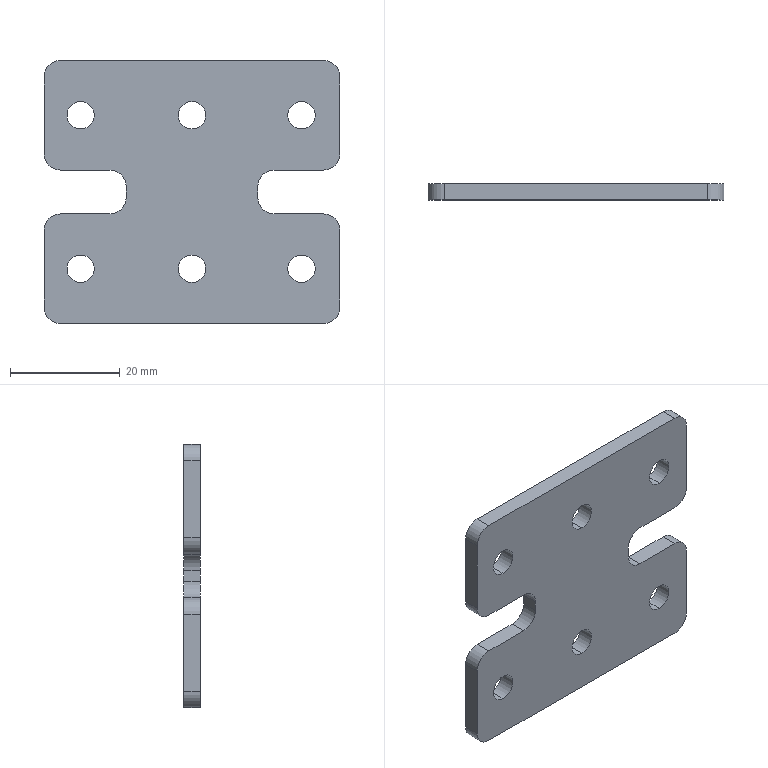Part | SolidWorks | features BaseBody 1 | 1 solid | 38 faces | box 54 x 3 x 48 mm | volume 6679 mm3 | cylinder 24 | plane 14 | commonest cylinder face diameters 5 x12 6 x12
STEP:
#1=CARTESIAN_POINT('',(20.,0.,11.5));
#2=VERTEX_POINT('',#1);
#3=CARTESIAN_POINT('',(20.,0.,16.5));
#4=VERTEX_POINT('',#3);
#5=CARTESIAN_POINT('',(20.,0.,14.));
#6=DIRECTION('',(0.,1.,0.));
#7=DIRECTION('',(0.,0.,1.));
#8=AXIS2_PLACEMENT_3D('',#5,#6,#7);
#9=CIRCLE('',#8,2.5);
#10=EDGE_CURVE('',#2,#4,#9,.T.);
#11=ORIENTED_EDGE('',*,*,#10,.F.);
#12=CARTESIAN_POINT('',(20.,3.,11.5));
#13=VERTEX_POINT('',#12);
#14=CARTESIAN_POINT('',(20.,0.,11.5));
#15=DIRECTION('',(0.,1.,0.));
#16=VECTOR('',#15,1000.);
#17=LINE('',#14,#16);
#18=EDGE_CURVE('',#2,#13,#17,.T.);
#19=ORIENTED_EDGE('',*,*,#18,.T.);
#20=CARTESIAN_POINT('',(20.,3.,16.5));
#21=VERTEX_POINT('',#20);
#22=CARTESIAN_POINT('',(20.,3.,14.));
#23=DIRECTION('',(0.,1.,0.));
#24=DIRECTION('',(0.,0.,1.));
#25=AXIS2_PLACEMENT_3D('',#22,#23,#24);
#26=CIRCLE('',#25,2.5);
#27=EDGE_CURVE('',#13,#21,#26,.T.);
#28=ORIENTED_EDGE('',*,*,#27,.T.);
#29=CARTESIAN_POINT('',(20.,0.,16.5));
#30=DIRECTION('',(0.,1.,0.));
#31=VECTOR('',#30,1000.);
#32=LINE('',#29,#31);
#33=EDGE_CURVE('',#4,#21,#32,.T.);
#34=ORIENTED_EDGE('',*,*,#33,.F.);
#35=EDGE_LOOP('',(#11,#19,#28,#34));
#36=FACE_OUTER_BOUND('',#35,.T.);
#37=CARTESIAN_POINT('',(20.,0.,14.));
#38=DIRECTION('',(0.,1.,0.));
#39=DIRECTION('',(0.,0.,1.));
#40=AXIS2_PLACEMENT_3D('',#37,#38,#39);
#41=CYLINDRICAL_SURFACE('',#40,2.5);
#42=ADVANCED_FACE('',(#36),#41,.F.);
#43=CARTESIAN_POINT('',(0.,0.,-16.5));
#44=VERTEX_POINT('',#43);
#45=CARTESIAN_POINT('',(0.,0.,-11.5));
#46=VERTEX_POINT('',#45);
#47=CARTESIAN_POINT('',(0.,0.,-14.));
#48=DIRECTION('',(0.,1.,0.));
#49=DIRECTION('',(0.,0.,1.));
#50=AXIS2_PLACEMENT_3D('',#47,#48,#49);
#51=CIRCLE('',#50,2.5);
#52=EDGE_CURVE('',#44,#46,#51,.T.);
#53=ORIENTED_EDGE('',*,*,#52,.F.);
#54=CARTESIAN_POINT('',(0.,3.,-16.5));
#55=VERTEX_POINT('',#54);
#56=CARTESIAN_POINT('',(0.,0.,-16.5));
#57=DIRECTION('',(0.,1.,0.));
#58=VECTOR('',#57,1000.);
#59=LINE('',#56,#58);
#60=EDGE_CURVE('',#44,#55,#59,.T.);
#61=ORIENTED_EDGE('',*,*,#60,.T.);
#62=CARTESIAN_POINT('',(0.,3.,-11.5));
#63=VERTEX_POINT('',#62);
#64=CARTESIAN_POINT('',(0.,3.,-14.));
#65=DIRECTION('',(0.,1.,0.));
#66=DIRECTION('',(0.,0.,1.));
#67=AXIS2_PLACEMENT_3D('',#64,#65,#66);
#68=CIRCLE('',#67,2.5);
#69=EDGE_CURVE('',#55,#63,#68,.T.);
#70=ORIENTED_EDGE('',*,*,#69,.T.);
#71=CARTESIAN_POINT('',(0.,0.,-11.5));
#72=DIRECTION('',(0.,1.,0.));
#73=VECTOR('',#72,1000.);
#74=LINE('',#71,#73);
#75=EDGE_CURVE('',#46,#63,#74,.T.);
#76=ORIENTED_EDGE('',*,*,#75,.F.);
#77=EDGE_LOOP('',(#53,#61,#70,#76));
#78=FACE_OUTER_BOUND('',#77,.T.);
#79=CARTESIAN_POINT('',(0.,0.,-14.));
#80=DIRECTION('',(0.,1.,0.));
#81=DIRECTION('',(0.,0.,1.));
#82=AXIS2_PLACEMENT_3D('',#79,#80,#81);
#83=CYLINDRICAL_SURFACE('',#82,2.5);
#84=ADVANCED_FACE('',(#78),#83,.F.);
#85=CARTESIAN_POINT('',(-20.32,0.,-16.5));
#86=VERTEX_POINT('',#85);
#87=CARTESIAN_POINT('',(-20.32,0.,-11.5));
#88=VERTEX_POINT('',#87);
#89=CARTESIAN_POINT('',(-20.32,0.,-14.));
#90=DIRECTION('',(0.,1.,0.));
#91=DIRECTION('',(0.,0.,1.));
#92=AXIS2_PLACEMENT_3D('',#89,#90,#91);
#93=CIRCLE('',#92,2.5);
#94=EDGE_CURVE('',#86,#88,#93,.T.);
#95=ORIENTED_EDGE('',*,*,#94,.F.);
#96=CARTESIAN_POINT('',(-20.32,3.,-16.5));
#97=VERTEX_POINT('',#96);
#98=CARTESIAN_POINT('',(-20.32,0.,-16.5));
#99=DIRECTION('',(0.,1.,0.));
#100=VECTOR('',#99,1000.);
#101=LINE('',#98,#100);
#102=EDGE_CURVE('',#86,#97,#101,.T.);
#103=ORIENTED_EDGE('',*,*,#102,.T.);
#104=CARTESIAN_POINT('',(-20.32,3.,-11.5));
#105=VERTEX_POINT('',#104);
#106=CARTESIAN_POINT('',(-20.32,3.,-14.));
#107=DIRECTION('',(0.,1.,0.));
#108=DIRECTION('',(0.,0.,1.));
#109=AXIS2_PLACEMENT_3D('',#106,#107,#108);
#110=CIRCLE('',#109,2.5);
#111=EDGE_CURVE('',#97,#105,#110,.T.);
#112=ORIENTED_EDGE('',*,*,#111,.T.);
#113=CARTESIAN_POINT('',(-20.32,0.,-11.5));
#114=DIRECTION('',(0.,1.,0.));
#115=VECTOR('',#114,1000.);
#116=LINE('',#113,#115);
#117=EDGE_CURVE('',#88,#105,#116,.T.);
#118=ORIENTED_EDGE('',*,*,#117,.F.);
#119=EDGE_LOOP('',(#95,#103,#112,#118));
#120=FACE_OUTER_BOUND('',#119,.T.);
#121=CARTESIAN_POINT('',(-20.32,0.,-14.));
#122=DIRECTION('',(0.,1.,0.));
#123=DIRECTION('',(0.,0.,1.));
#124=AXIS2_PLACEMENT_3D('',#121,#122,#123);
#125=CYLINDRICAL_SURFACE('',#124,2.5);
#126=ADVANCED_FACE('',(#120),#125,.F.);
#127=CARTESIAN_POINT('',(0.,0.,11.5));
#128=VERTEX_POINT('',#127);
#129=CARTESIAN_POINT('',(0.,0.,16.5));
#130=VERTEX_POINT('',#129);
#131=CARTESIAN_POINT('',(0.,0.,14.));
#132=DIRECTION('',(0.,1.,0.));
#133=DIRECTION('',(0.,0.,1.));
#134=AXIS2_PLACEMENT_3D('',#131,#132,#133);
#135=CIRCLE('',#134,2.5);
#136=EDGE_CURVE('',#128,#130,#135,.T.);
#137=ORIENTED_EDGE('',*,*,#136,.F.);
#138=CARTESIAN_POINT('',(0.,3.,11.5));
#139=VERTEX_POINT('',#138);
#140=CARTESIAN_POINT('',(0.,0.,11.5));
#141=DIRECTION('',(0.,1.,0.));
#142=VECTOR('',#141,1000.);
#143=LINE('',#140,#142);
#144=EDGE_CURVE('',#128,#139,#143,.T.);
#145=ORIENTED_EDGE('',*,*,#144,.T.);
#146=CARTESIAN_POINT('',(0.,3.,16.5));
#147=VERTEX_POINT('',#146);
#148=CARTESIAN_POINT('',(0.,3.,14.));
#149=DIRECTION('',(0.,1.,0.));
#150=DIRECTION('',(0.,0.,1.));
#151=AXIS2_PLACEMENT_3D('',#148,#149,#150);
#152=CIRCLE('',#151,2.5);
#153=EDGE_CURVE('',#139,#147,#152,.T.);
#154=ORIENTED_EDGE('',*,*,#153,.T.);
#155=CARTESIAN_POINT('',(0.,0.,16.5));
#156=DIRECTION('',(0.,1.,0.));
#157=VECTOR('',#156,1000.);
#158=LINE('',#155,#157);
#159=EDGE_CURVE('',#130,#147,#158,.T.);
#160=ORIENTED_EDGE('',*,*,#159,.F.);
#161=EDGE_LOOP('',(#137,#145,#154,#160));
#162=FACE_OUTER_BOUND('',#161,.T.);
#163=CARTESIAN_POINT('',(0.,0.,14.));
#164=DIRECTION('',(0.,1.,0.));
#165=DIRECTION('',(0.,0.,1.));
#166=AXIS2_PLACEMENT_3D('',#163,#164,#165);
#167=CYLINDRICAL_SURFACE('',#166,2.5);
#168=ADVANCED_FACE('',(#162),#167,.F.);
#169=CARTESIAN_POINT('',(-20.32,0.,11.5));
#170=VERTEX_POINT('',#169);
#171=CARTESIAN_POINT('',(-20.32,0.,16.5));
#172=VERTEX_POINT('',#171);
#173=CARTESIAN_POINT('',(-20.32,0.,14.));
#174=DIRECTION('',(0.,1.,0.));
#175=DIRECTION('',(0.,0.,1.));
#176=AXIS2_PLACEMENT_3D('',#173,#174,#175);
#177=CIRCLE('',#176,2.5);
#178=EDGE_CURVE('',#170,#172,#177,.T.);
#179=ORIENTED_EDGE('',*,*,#178,.F.);
#180=CARTESIAN_POINT('',(-20.32,3.,11.5));
#181=VERTEX_POINT('',#180);
#182=CARTESIAN_POINT('',(-20.32,0.,11.5));
#183=DIRECTION('',(0.,1.,0.));
#184=VECTOR('',#183,1000.);
#185=LINE('',#182,#184);
#186=EDGE_CURVE('',#170,#181,#185,.T.);
#187=ORIENTED_EDGE('',*,*,#186,.T.);
#188=CARTESIAN_POINT('',(-20.32,3.,16.5));
#189=VERTEX_POINT('',#188);
#190=CARTESIAN_POINT('',(-20.32,3.,14.));
#191=DIRECTION('',(0.,1.,0.));
#192=DIRECTION('',(0.,0.,1.));
#193=AXIS2_PLACEMENT_3D('',#190,#191,#192);
#194=CIRCLE('',#193,2.5);
#195=EDGE_CURVE('',#181,#189,#194,.T.);
#196=ORIENTED_EDGE('',*,*,#195,.T.);
#197=CARTESIAN_POINT('',(-20.32,0.,16.5));
#198=DIRECTION('',(0.,1.,0.));
#199=VECTOR('',#198,1000.);
#200=LINE('',#197,#199);
#201=EDGE_CURVE('',#172,#189,#200,.T.);
#202=ORIENTED_EDGE('',*,*,#201,.F.);
#203=EDGE_LOOP('',(#179,#187,#196,#202));
#204=FACE_OUTER_BOUND('',#203,.T.);
#205=CARTESIAN_POINT('',(-20.32,0.,14.));
#206=DIRECTION('',(0.,1.,0.));
#207=DIRECTION('',(0.,0.,1.));
#208=AXIS2_PLACEMENT_3D('',#205,#206,#207);
#209=CYLINDRICAL_SURFACE('',#208,2.5);
#210=ADVANCED_FACE('',(#204),#209,.F.);
#211=CARTESIAN_POINT('',(20.,0.,-16.5));
#212=VERTEX_POINT('',#211);
#213=CARTESIAN_POINT('',(20.,0.,-11.5));
#214=VERTEX_POINT('',#213);
#215=CARTESIAN_POINT('',(20.,0.,-14.));
#216=DIRECTION('',(0.,1.,0.));
#217=DIRECTION('',(0.,0.,1.));
#218=AXIS2_PLACEMENT_3D('',#215,#216,#217);
#219=CIRCLE('',#218,2.5);
#220=EDGE_CURVE('',#212,#214,#219,.T.);
#221=ORIENTED_EDGE('',*,*,#220,.F.);
#222=CARTESIAN_POINT('',(20.,3.,-16.5));
#223=VERTEX_POINT('',#222);
#224=CARTESIAN_POINT('',(20.,0.,-16.5));
#225=DIRECTION('',(0.,1.,0.));
#226=VECTOR('',#225,1000.);
#227=LINE('',#224,#226);
#228=EDGE_CURVE('',#212,#223,#227,.T.);
#229=ORIENTED_EDGE('',*,*,#228,.T.);
#230=CARTESIAN_POINT('',(20.,3.,-11.5));
#231=VERTEX_POINT('',#230);
#232=CARTESIAN_POINT('',(20.,3.,-14.));
#233=DIRECTION('',(0.,1.,0.));
#234=DIRECTION('',(0.,0.,1.));
#235=AXIS2_PLACEMENT_3D('',#232,#233,#234);
#236=CIRCLE('',#235,2.5);
#237=EDGE_CURVE('',#223,#231,#236,.T.);
#238=ORIENTED_EDGE('',*,*,#237,.T.);
#239=CARTESIAN_POINT('',(20.,0.,-11.5));
#240=DIRECTION('',(0.,1.,0.));
#241=VECTOR('',#240,1000.);
#242=LINE('',#239,#241);
#243=EDGE_CURVE('',#214,#231,#242,.T.);
#244=ORIENTED_EDGE('',*,*,#243,.F.);
#245=EDGE_LOOP('',(#221,#229,#238,#244));
#246=FACE_OUTER_BOUND('',#245,.T.);
#247=CARTESIAN_POINT('',(20.,0.,-14.));
#248=DIRECTION('',(0.,1.,0.));
#249=DIRECTION('',(0.,0.,1.));
#250=AXIS2_PLACEMENT_3D('',#247,#248,#249);
#251=CYLINDRICAL_SURFACE('',#250,2.5);
#252=ADVANCED_FACE('',(#246),#251,.F.);
#253=CARTESIAN_POINT('',(24.,3.,4.));
#254=VERTEX_POINT('',#253);
#255=CARTESIAN_POINT('',(27.,3.,7.));
#256=VERTEX_POINT('',#255);
#257=CARTESIAN_POINT('',(24.,3.,7.));
#258=DIRECTION('',(0.,-1.,0.));
#259=DIRECTION('',(0.,0.,1.));
#260=AXIS2_PLACEMENT_3D('',#257,#258,#259);
#261=CIRCLE('',#260,3.);
#262=EDGE_CURVE('',#254,#256,#261,.T.);
#263=ORIENTED_EDGE('',*,*,#262,.F.);
#264=CARTESIAN_POINT('',(15.,3.,4.));
#265=VERTEX_POINT('',#264);
#266=CARTESIAN_POINT('',(0.,3.,4.));
#267=DIRECTION('',(1.,0.,0.));
#268=VECTOR('',#267,1000.);
#269=LINE('',#266,#268);
#270=EDGE_CURVE('',#265,#254,#269,.T.);
#271=ORIENTED_EDGE('',*,*,#270,.F.);
#272=CARTESIAN_POINT('',(12.,3.,1.));
#273=VERTEX_POINT('',#272);
#274=CARTESIAN_POINT('',(15.,3.,1.));
#275=DIRECTION('',(0.,1.,0.));
#276=DIRECTION('',(0.,0.,-1.));
#277=AXIS2_PLACEMENT_3D('',#274,#275,#276);
#278=CIRCLE('',#277,3.);
#279=EDGE_CURVE('',#273,#265,#278,.T.);
#280=ORIENTED_EDGE('',*,*,#279,.F.);
#281=CARTESIAN_POINT('',(12.,3.,-1.));
#282=VERTEX_POINT('',#281);
#283=CARTESIAN_POINT('',(12.,3.,0.));
#284=DIRECTION('',(0.,0.,1.));
#285=VECTOR('',#284,1000.);
#286=LINE('',#283,#285);
#287=EDGE_CURVE('',#282,#273,#286,.T.);
#288=ORIENTED_EDGE('',*,*,#287,.F.);
#289=CARTESIAN_POINT('',(15.,3.,-4.));
#290=VERTEX_POINT('',#289);
#291=CARTESIAN_POINT('',(15.,3.,-1.));
#292=DIRECTION('',(0.,1.,0.));
#293=DIRECTION('',(0.,0.,-1.));
#294=AXIS2_PLACEMENT_3D('',#291,#292,#293);
#295=CIRCLE('',#294,3.);
#296=EDGE_CURVE('',#290,#282,#295,.T.);
#297=ORIENTED_EDGE('',*,*,#296,.F.);
#298=CARTESIAN_POINT('',(24.,3.,-4.));
#299=VERTEX_POINT('',#298);
#300=CARTESIAN_POINT('',(0.,3.,-4.));
#301=DIRECTION('',(-1.,0.,0.));
#302=VECTOR('',#301,1000.);
#303=LINE('',#300,#302);
#304=EDGE_CURVE('',#299,#290,#303,.T.);
#305=ORIENTED_EDGE('',*,*,#304,.F.);
#306=CARTESIAN_POINT('',(27.,3.,-7.));
#307=VERTEX_POINT('',#306);
#308=CARTESIAN_POINT('',(24.,3.,-7.));
#309=DIRECTION('',(0.,-1.,0.));
#310=DIRECTION('',(0.,0.,-1.));
#311=AXIS2_PLACEMENT_3D('',#308,#309,#310);
#312=CIRCLE('',#311,3.);
#313=EDGE_CURVE('',#307,#299,#312,.T.);
#314=ORIENTED_EDGE('',*,*,#313,.F.);
#315=CARTESIAN_POINT('',(27.,3.,-21.));
#316=VERTEX_POINT('',#315);
#317=CARTESIAN_POINT('',(27.,3.,0.));
#318=DIRECTION('',(0.,0.,1.));
#319=VECTOR('',#318,1000.);
#320=LINE('',#317,#319);
#321=EDGE_CURVE('',#316,#307,#320,.T.);
#322=ORIENTED_EDGE('',*,*,#321,.F.);
#323=CARTESIAN_POINT('',(24.,3.,-24.));
#324=VERTEX_POINT('',#323);
#325=CARTESIAN_POINT('',(24.,3.,-21.));
#326=DIRECTION('',(0.,-1.,0.));
#327=DIRECTION('',(0.,0.,-1.));
#328=AXIS2_PLACEMENT_3D('',#325,#326,#327);
#329=CIRCLE('',#328,3.);
#330=EDGE_CURVE('',#324,#316,#329,.T.);
#331=ORIENTED_EDGE('',*,*,#330,.F.);
#332=CARTESIAN_POINT('',(-24.,3.,-24.));
#333=VERTEX_POINT('',#332);
#334=CARTESIAN_POINT('',(0.,3.,-24.));
#335=DIRECTION('',(1.,0.,0.));
#336=VECTOR('',#335,1000.);
#337=LINE('',#334,#336);
#338=EDGE_CURVE('',#333,#324,#337,.T.);
#339=ORIENTED_EDGE('',*,*,#338,.F.);
#340=CARTESIAN_POINT('',(-27.,3.,-21.));
#341=VERTEX_POINT('',#340);
#342=CARTESIAN_POINT('',(-24.,3.,-21.));
#343=DIRECTION('',(0.,-1.,0.));
#344=DIRECTION('',(0.,0.,-1.));
#345=AXIS2_PLACEMENT_3D('',#342,#343,#344);
#346=CIRCLE('',#345,3.);
#347=EDGE_CURVE('',#341,#333,#346,.T.);
#348=ORIENTED_EDGE('',*,*,#347,.F.);
#349=CARTESIAN_POINT('',(-27.,3.,-7.));
#350=VERTEX_POINT('',#349);
#351=CARTESIAN_POINT('',(-27.,3.,0.));
#352=DIRECTION('',(0.,0.,-1.));
#353=VECTOR('',#352,1000.);
#354=LINE('',#351,#353);
#355=EDGE_CURVE('',#350,#341,#354,.T.);
#356=ORIENTED_EDGE('',*,*,#355,.F.);
#357=CARTESIAN_POINT('',(-24.,3.,-4.));
#358=VERTEX_POINT('',#357);
#359=CARTESIAN_POINT('',(-24.,3.,-7.));
#360=DIRECTION('',(0.,-1.,0.));
#361=DIRECTION('',(0.,0.,1.));
#362=AXIS2_PLACEMENT_3D('',#359,#360,#361);
#363=CIRCLE('',#362,3.);
#364=EDGE_CURVE('',#358,#350,#363,.T.);
#365=ORIENTED_EDGE('',*,*,#364,.F.);
#366=CARTESIAN_POINT('',(-15.,3.,-4.));
#367=VERTEX_POINT('',#366);
#368=CARTESIAN_POINT('',(0.,3.,-4.));
#369=DIRECTION('',(-1.,0.,0.));
#370=VECTOR('',#369,1000.);
#371=LINE('',#368,#370);
#372=EDGE_CURVE('',#367,#358,#371,.T.);
#373=ORIENTED_EDGE('',*,*,#372,.F.);
#374=CARTESIAN_POINT('',(-12.,3.,-1.));
#375=VERTEX_POINT('',#374);
#376=CARTESIAN_POINT('',(-15.,3.,-1.));
#377=DIRECTION('',(0.,1.,0.));
#378=DIRECTION('',(0.,0.,-1.));
#379=AXIS2_PLACEMENT_3D('',#376,#377,#378);
#380=CIRCLE('',#379,3.);
#381=EDGE_CURVE('',#375,#367,#380,.T.);
#382=ORIENTED_EDGE('',*,*,#381,.F.);
#383=CARTESIAN_POINT('',(-12.,3.,1.));
#384=VERTEX_POINT('',#383);
#385=CARTESIAN_POINT('',(-12.,3.,0.));
#386=DIRECTION('',(0.,0.,-1.));
#387=VECTOR('',#386,1000.);
#388=LINE('',#385,#387);
#389=EDGE_CURVE('',#384,#375,#388,.T.);
#390=ORIENTED_EDGE('',*,*,#389,.F.);
#391=CARTESIAN_POINT('',(-15.,3.,4.));
#392=VERTEX_POINT('',#391);
#393=CARTESIAN_POINT('',(-15.,3.,1.));
#394=DIRECTION('',(0.,1.,0.));
#395=DIRECTION('',(0.,0.,-1.));
#396=AXIS2_PLACEMENT_3D('',#393,#394,#395);
#397=CIRCLE('',#396,3.);
#398=EDGE_CURVE('',#392,#384,#397,.T.);
#399=ORIENTED_EDGE('',*,*,#398,.F.);
#400=CARTESIAN_POINT('',(-24.,3.,4.));
#401=VERTEX_POINT('',#400);
#402=CARTESIAN_POINT('',(0.,3.,4.));
#403=DIRECTION('',(1.,0.,0.));
#404=VECTOR('',#403,1000.);
#405=LINE('',#402,#404);
#406=EDGE_CURVE('',#401,#392,#405,.T.);
#407=ORIENTED_EDGE('',*,*,#406,.F.);
#408=CARTESIAN_POINT('',(-27.,3.,7.));
#409=VERTEX_POINT('',#408);
#410=CARTESIAN_POINT('',(-24.,3.,7.));
#411=DIRECTION('',(0.,-1.,0.));
#412=DIRECTION('',(0.,0.,-1.));
#413=AXIS2_PLACEMENT_3D('',#410,#411,#412);
#414=CIRCLE('',#413,3.);
#415=EDGE_CURVE('',#409,#401,#414,.T.);
#416=ORIENTED_EDGE('',*,*,#415,.F.);
#417=CARTESIAN_POINT('',(-27.,3.,21.));
#418=VERTEX_POINT('',#417);
#419=CARTESIAN_POINT('',(-27.,3.,0.));
#420=DIRECTION('',(0.,0.,-1.));
#421=VECTOR('',#420,1000.);
#422=LINE('',#419,#421);
#423=EDGE_CURVE('',#418,#409,#422,.T.);
#424=ORIENTED_EDGE('',*,*,#423,.F.);
#425=CARTESIAN_POINT('',(-24.,3.,24.));
#426=VERTEX_POINT('',#425);
#427=CARTESIAN_POINT('',(-24.,3.,21.));
#428=DIRECTION('',(0.,-1.,0.));
#429=DIRECTION('',(0.,0.,-1.));
#430=AXIS2_PLACEMENT_3D('',#427,#428,#429);
#431=CIRCLE('',#430,3.);
#432=EDGE_CURVE('',#426,#418,#431,.T.);
#433=ORIENTED_EDGE('',*,*,#432,.F.);
#434=CARTESIAN_POINT('',(24.,3.,24.));
#435=VERTEX_POINT('',#434);
#436=CARTESIAN_POINT('',(0.,3.,24.));
#437=DIRECTION('',(-1.,0.,0.));
#438=VECTOR('',#437,1000.);
#439=LINE('',#436,#438);
#440=EDGE_CURVE('',#435,#426,#439,.T.);
#441=ORIENTED_EDGE('',*,*,#440,.F.);
#442=CARTESIAN_POINT('',(27.,3.,21.));
#443=VERTEX_POINT('',#442);
#444=CARTESIAN_POINT('',(24.,3.,21.));
#445=DIRECTION('',(0.,-1.,0.));
#446=DIRECTION('',(0.,0.,-1.));
#447=AXIS2_PLACEMENT_3D('',#444,#445,#446);
#448=CIRCLE('',#447,3.);
#449=EDGE_CURVE('',#443,#435,#448,.T.);
#450=ORIENTED_EDGE('',*,*,#449,.F.);
#451=CARTESIAN_POINT('',(27.,3.,0.));
#452=DIRECTION('',(0.,0.,1.));
#453=VECTOR('',#452,1000.);
#454=LINE('',#451,#453);
#455=EDGE_CURVE('',#256,#443,#454,.T.);
#456=ORIENTED_EDGE('',*,*,#455,.F.);
#457=EDGE_LOOP('',(#263,#271,#280,#288,#297,#305,#314,#322,#331,#339,#348,#356,#365,#373,#382,#390,#399,#407,#416,#424,#433,#441,#450,#456));
#458=FACE_OUTER_BOUND('',#457,.T.);
#459=CARTESIAN_POINT('',(20.,3.,14.));
#460=DIRECTION('',(0.,1.,0.));
#461=DIRECTION('',(0.,0.,1.));
#462=AXIS2_PLACEMENT_3D('',#459,#460,#461);
#463=CIRCLE('',#462,2.5);
#464=EDGE_CURVE('',#21,#13,#463,.T.);
#465=ORIENTED_EDGE('',*,*,#464,.F.);
#466=ORIENTED_EDGE('',*,*,#27,.F.);
#467=EDGE_LOOP('',(#465,#466));
#468=FACE_BOUND('',#467,.T.);
#469=CARTESIAN_POINT('',(0.,3.,-14.));
#470=DIRECTION('',(0.,1.,0.));
#471=DIRECTION('',(0.,0.,1.));
#472=AXIS2_PLACEMENT_3D('',#469,#470,#471);
#473=CIRCLE('',#472,2.5);
#474=EDGE_CURVE('',#63,#55,#473,.T.);
#475=ORIENTED_EDGE('',*,*,#474,.F.);
#476=ORIENTED_EDGE('',*,*,#69,.F.);
#477=EDGE_LOOP('',(#475,#476));
#478=FACE_BOUND('',#477,.T.);
#479=CARTESIAN_POINT('',(-20.32,3.,-14.));
#480=DIRECTION('',(0.,1.,0.));
#481=DIRECTION('',(0.,0.,1.));
#482=AXIS2_PLACEMENT_3D('',#479,#480,#481);
#483=CIRCLE('',#482,2.5);
#484=EDGE_CURVE('',#105,#97,#483,.T.);
#485=ORIENTED_EDGE('',*,*,#484,.F.);
#486=ORIENTED_EDGE('',*,*,#111,.F.);
#487=EDGE_LOOP('',(#485,#486));
#488=FACE_BOUND('',#487,.T.);
#489=CARTESIAN_POINT('',(0.,3.,14.));
#490=DIRECTION('',(0.,1.,0.));
#491=DIRECTION('',(0.,0.,1.));
#492=AXIS2_PLACEMENT_3D('',#489,#490,#491);
#493=CIRCLE('',#492,2.5);
#494=EDGE_CURVE('',#147,#139,#493,.T.);
#495=ORIENTED_EDGE('',*,*,#494,.F.);
#496=ORIENTED_EDGE('',*,*,#153,.F.);
#497=EDGE_LOOP('',(#495,#496));
#498=FACE_BOUND('',#497,.T.);
#499=CARTESIAN_POINT('',(-20.32,3.,14.));
#500=DIRECTION('',(0.,1.,0.));
#501=DIRECTION('',(0.,0.,1.));
#502=AXIS2_PLACEMENT_3D('',#499,#500,#501);
#503=CIRCLE('',#502,2.5);
#504=EDGE_CURVE('',#189,#181,#503,.T.);
#505=ORIENTED_EDGE('',*,*,#504,.F.);
#506=ORIENTED_EDGE('',*,*,#195,.F.);
#507=EDGE_LOOP('',(#505,#506));
#508=FACE_BOUND('',#507,.T.);
#509=CARTESIAN_POINT('',(20.,3.,-14.));
#510=DIRECTION('',(0.,1.,0.));
#511=DIRECTION('',(0.,0.,1.));
#512=AXIS2_PLACEMENT_3D('',#509,#510,#511);
#513=CIRCLE('',#512,2.5);
#514=EDGE_CURVE('',#231,#223,#513,.T.);
#515=ORIENTED_EDGE('',*,*,#514,.F.);
#516=ORIENTED_EDGE('',*,*,#237,.F.);
#517=EDGE_LOOP('',(#515,#516));
#518=FACE_BOUND('',#517,.T.);
#519=CARTESIAN_POINT('',(0.,3.,0.));
#520=DIRECTION('',(0.,-1.,0.));
#521=DIRECTION('',(0.,0.,-1.));
#522=AXIS2_PLACEMENT_3D('',#519,#520,#521);
#523=PLANE('',#522);
#524=ADVANCED_FACE('',(#458,#468,#478,#488,#498,#508,#518),#523,.F.);
#525=CARTESIAN_POINT('',(27.,0.,7.));
#526=VERTEX_POINT('',#525);
#527=CARTESIAN_POINT('',(27.,3.,7.));
#528=DIRECTION('',(0.,-1.,0.));
#529=VECTOR('',#528,1000.);
#530=LINE('',#527,#529);
#531=EDGE_CURVE('',#256,#526,#530,.T.);
#532=ORIENTED_EDGE('',*,*,#531,.F.);
#533=ORIENTED_EDGE('',*,*,#455,.T.);
#534=CARTESIAN_POINT('',(27.,0.,21.));
#535=VERTEX_POINT('',#534);
#536=CARTESIAN_POINT('',(27.,3.,21.));
#537=DIRECTION('',(0.,1.,0.));
#538=VECTOR('',#537,1000.);
#539=LINE('',#536,#538);
#540=EDGE_CURVE('',#535,#443,#539,.T.);
#541=ORIENTED_EDGE('',*,*,#540,.F.);
#542=CARTESIAN_POINT('',(27.,0.,24.));
#543=DIRECTION('',(0.,0.,1.));
#544=VECTOR('',#543,1000.);
#545=LINE('',#542,#544);
#546=EDGE_CURVE('',#526,#535,#545,.T.);
#547=ORIENTED_EDGE('',*,*,#546,.F.);
#548=EDGE_LOOP('',(#532,#533,#541,#547));
#549=FACE_OUTER_BOUND('',#548,.T.);
#550=CARTESIAN_POINT('',(27.,3.,24.));
#551=DIRECTION('',(-1.,0.,0.));
#552=DIRECTION('',(0.,0.,1.));
#553=AXIS2_PLACEMENT_3D('',#550,#551,#552);
#554=PLANE('',#553);
#555=ADVANCED_FACE('',(#549),#554,.F.);
#556=ORIENTED_EDGE('',*,*,#262,.T.);
#557=ORIENTED_EDGE('',*,*,#531,.T.);
#558=CARTESIAN_POINT('',(24.,0.,4.));
#559=VERTEX_POINT('',#558);
#560=CARTESIAN_POINT('',(24.,0.,7.));
#561=DIRECTION('',(0.,1.,0.));
#562=DIRECTION('',(0.,0.,1.));
#563=AXIS2_PLACEMENT_3D('',#560,#561,#562);
#564=CIRCLE('',#563,3.);
#565=EDGE_CURVE('',#526,#559,#564,.T.);
#566=ORIENTED_EDGE('',*,*,#565,.T.);
#567=CARTESIAN_POINT('',(24.,3.,4.));
#568=DIRECTION('',(0.,1.,0.));
#569=VECTOR('',#568,1000.);
#570=LINE('',#567,#569);
#571=EDGE_CURVE('',#559,#254,#570,.T.);
#572=ORIENTED_EDGE('',*,*,#571,.T.);
#573=EDGE_LOOP('',(#556,#557,#566,#572));
#574=FACE_OUTER_BOUND('',#573,.T.);
#575=CARTESIAN_POINT('',(24.,3.,7.));
#576=DIRECTION('',(0.,1.,0.));
#577=DIRECTION('',(0.,0.,1.));
#578=AXIS2_PLACEMENT_3D('',#575,#576,#577);
#579=CYLINDRICAL_SURFACE('',#578,3.);
#580=ADVANCED_FACE('',(#574),#579,.T.);
#581=CARTESIAN_POINT('',(15.,0.,4.));
#582=VERTEX_POINT('',#581);
#583=CARTESIAN_POINT('',(15.,0.,4.));
#584=DIRECTION('',(0.,-1.,0.));
#585=VECTOR('',#584,1000.);
#586=LINE('',#583,#585);
#587=EDGE_CURVE('',#265,#582,#586,.T.);
#588=ORIENTED_EDGE('',*,*,#587,.F.);
#589=ORIENTED_EDGE('',*,*,#270,.T.);
#590=ORIENTED_EDGE('',*,*,#571,.F.);
#591=CARTESIAN_POINT('',(42.,0.,4.));
#592=DIRECTION('',(1.,0.,0.));
#593=VECTOR('',#592,1000.);
#594=LINE('',#591,#593);
#595=EDGE_CURVE('',#582,#559,#594,.T.);
#596=ORIENTED_EDGE('',*,*,#595,.F.);
#597=EDGE_LOOP('',(#588,#589,#590,#596));
#598=FACE_OUTER_BOUND('',#597,.T.);
#599=CARTESIAN_POINT('',(42.,0.,4.));
#600=DIRECTION('',(0.,0.,1.));
#601=DIRECTION('',(1.,0.,0.));
#602=AXIS2_PLACEMENT_3D('',#599,#600,#601);
#603=PLANE('',#602);
#604=ADVANCED_FACE('',(#598),#603,.F.);
#605=CARTESIAN_POINT('',(12.,0.,1.));
#606=VERTEX_POINT('',#605);
#607=CARTESIAN_POINT('',(12.,0.,1.));
#608=DIRECTION('',(0.,-1.,0.));
#609=VECTOR('',#608,1000.);
#610=LINE('',#607,#609);
#611=EDGE_CURVE('',#273,#606,#610,.T.);
#612=ORIENTED_EDGE('',*,*,#611,.F.);
#613=ORIENTED_EDGE('',*,*,#279,.T.);
#614=ORIENTED_EDGE('',*,*,#587,.T.);
#615=CARTESIAN_POINT('',(15.,0.,1.));
#616=DIRECTION('',(0.,1.,0.));
#617=DIRECTION('',(0.,0.,-1.));
#618=AXIS2_PLACEMENT_3D('',#615,#616,#617);
#619=CIRCLE('',#618,3.);
#620=EDGE_CURVE('',#606,#582,#619,.T.);
#621=ORIENTED_EDGE('',*,*,#620,.F.);
#622=EDGE_LOOP('',(#612,#613,#614,#621));
#623=FACE_OUTER_BOUND('',#622,.T.);
#624=CARTESIAN_POINT('',(15.,0.,1.));
#625=DIRECTION('',(0.,-1.,0.));
#626=DIRECTION('',(0.,0.,-1.));
#627=AXIS2_PLACEMENT_3D('',#624,#625,#626);
#628=CYLINDRICAL_SURFACE('',#627,3.);
#629=ADVANCED_FACE('',(#623),#628,.F.);
#630=ORIENTED_EDGE('',*,*,#611,.T.);
#631=CARTESIAN_POINT('',(12.,0.,-1.));
#632=VERTEX_POINT('',#631);
#633=CARTESIAN_POINT('',(12.,0.,4.));
#634=DIRECTION('',(0.,0.,1.));
#635=VECTOR('',#634,1000.);
#636=LINE('',#633,#635);
#637=EDGE_CURVE('',#632,#606,#636,.T.);
#638=ORIENTED_EDGE('',*,*,#637,.F.);
#639=CARTESIAN_POINT('',(12.,0.,-1.));
#640=DIRECTION('',(0.,-1.,0.));
#641=VECTOR('',#640,1000.);
#642=LINE('',#639,#641);
#643=EDGE_CURVE('',#282,#632,#642,.T.);
#644=ORIENTED_EDGE('',*,*,#643,.F.);
#645=ORIENTED_EDGE('',*,*,#287,.T.);
#646=EDGE_LOOP('',(#630,#638,#644,#645));
#647=FACE_OUTER_BOUND('',#646,.T.);
#648=CARTESIAN_POINT('',(12.,0.,4.));
#649=DIRECTION('',(-1.,0.,0.));
#650=DIRECTION('',(0.,0.,1.));
#651=AXIS2_PLACEMENT_3D('',#648,#649,#650);
#652=PLANE('',#651);
#653=ADVANCED_FACE('',(#647),#652,.F.);
#654=CARTESIAN_POINT('',(15.,0.,-4.));
#655=VERTEX_POINT('',#654);
#656=CARTESIAN_POINT('',(15.,0.,-4.));
#657=DIRECTION('',(0.,-1.,0.));
#658=VECTOR('',#657,1000.);
#659=LINE('',#656,#658);
#660=EDGE_CURVE('',#290,#655,#659,.T.);
#661=ORIENTED_EDGE('',*,*,#660,.F.);
#662=ORIENTED_EDGE('',*,*,#296,.T.);
#663=ORIENTED_EDGE('',*,*,#643,.T.);
#664=CARTESIAN_POINT('',(15.,0.,-1.));
#665=DIRECTION('',(0.,1.,0.));
#666=DIRECTION('',(0.,0.,-1.));
#667=AXIS2_PLACEMENT_3D('',#664,#665,#666);
#668=CIRCLE('',#667,3.);
#669=EDGE_CURVE('',#655,#632,#668,.T.);
#670=ORIENTED_EDGE('',*,*,#669,.F.);
#671=EDGE_LOOP('',(#661,#662,#663,#670));
#672=FACE_OUTER_BOUND('',#671,.T.);
#673=CARTESIAN_POINT('',(15.,0.,-1.));
#674=DIRECTION('',(0.,-1.,0.));
#675=DIRECTION('',(0.,0.,-1.));
#676=AXIS2_PLACEMENT_3D('',#673,#674,#675);
#677=CYLINDRICAL_SURFACE('',#676,3.);
#678=ADVANCED_FACE('',(#672),#677,.F.);
#679=CARTESIAN_POINT('',(24.,0.,-4.));
#680=VERTEX_POINT('',#679);
#681=CARTESIAN_POINT('',(24.,0.,-4.));
#682=DIRECTION('',(0.,-1.,0.));
#683=VECTOR('',#682,1000.);
#684=LINE('',#681,#683);
#685=EDGE_CURVE('',#299,#680,#684,.T.);
#686=ORIENTED_EDGE('',*,*,#685,.F.);
#687=ORIENTED_EDGE('',*,*,#304,.T.);
#688=ORIENTED_EDGE('',*,*,#660,.T.);
#689=CARTESIAN_POINT('',(42.,0.,-4.));
#690=DIRECTION('',(-1.,0.,0.));
#691=VECTOR('',#690,1000.);
#692=LINE('',#689,#691);
#693=EDGE_CURVE('',#680,#655,#692,.T.);
#694=ORIENTED_EDGE('',*,*,#693,.F.);
#695=EDGE_LOOP('',(#686,#687,#688,#694));
#696=FACE_OUTER_BOUND('',#695,.T.);
#697=CARTESIAN_POINT('',(42.,0.,-4.));
#698=DIRECTION('',(0.,0.,-1.));
#699=DIRECTION('',(-1.,0.,0.));
#700=AXIS2_PLACEMENT_3D('',#697,#698,#699);
#701=PLANE('',#700);
#702=ADVANCED_FACE('',(#696),#701,.F.);
#703=CARTESIAN_POINT('',(27.,0.,-7.));
#704=VERTEX_POINT('',#703);
#705=CARTESIAN_POINT('',(24.,0.,-7.));
#706=DIRECTION('',(0.,1.,0.));
#707=DIRECTION('',(0.,0.,-1.));
#708=AXIS2_PLACEMENT_3D('',#705,#706,#707);
#709=CIRCLE('',#708,3.);
#710=EDGE_CURVE('',#680,#704,#709,.T.);
#711=ORIENTED_EDGE('',*,*,#710,.T.);
#712=CARTESIAN_POINT('',(27.,3.,-7.));
#713=DIRECTION('',(0.,1.,0.));
#714=VECTOR('',#713,1000.);
#715=LINE('',#712,#714);
#716=EDGE_CURVE('',#704,#307,#715,.T.);
#717=ORIENTED_EDGE('',*,*,#716,.T.);
#718=ORIENTED_EDGE('',*,*,#313,.T.);
#719=ORIENTED_EDGE('',*,*,#685,.T.);
#720=EDGE_LOOP('',(#711,#717,#718,#719));
#721=FACE_OUTER_BOUND('',#720,.T.);
#722=CARTESIAN_POINT('',(24.,3.,-7.));
#723=DIRECTION('',(0.,-1.,0.));
#724=DIRECTION('',(0.,0.,-1.));
#725=AXIS2_PLACEMENT_3D('',#722,#723,#724);
#726=CYLINDRICAL_SURFACE('',#725,3.);
#727=ADVANCED_FACE('',(#721),#726,.T.);
#728=ORIENTED_EDGE('',*,*,#716,.F.);
#729=CARTESIAN_POINT('',(27.,0.,-21.));
#730=VERTEX_POINT('',#729);
#731=CARTESIAN_POINT('',(27.,0.,24.));
#732=DIRECTION('',(0.,0.,1.));
#733=VECTOR('',#732,1000.);
#734=LINE('',#731,#733);
#735=EDGE_CURVE('',#730,#704,#734,.T.);
#736=ORIENTED_EDGE('',*,*,#735,.F.);
#737=CARTESIAN_POINT('',(27.,3.,-21.));
#738=DIRECTION('',(0.,-1.,0.));
#739=VECTOR('',#738,1000.);
#740=LINE('',#737,#739);
#741=EDGE_CURVE('',#316,#730,#740,.T.);
#742=ORIENTED_EDGE('',*,*,#741,.F.);
#743=ORIENTED_EDGE('',*,*,#321,.T.);
#744=EDGE_LOOP('',(#728,#736,#742,#743));
#745=FACE_OUTER_BOUND('',#744,.T.);
#746=CARTESIAN_POINT('',(27.,3.,24.));
#747=DIRECTION('',(-1.,0.,0.));
#748=DIRECTION('',(0.,0.,1.));
#749=AXIS2_PLACEMENT_3D('',#746,#747,#748);
#750=PLANE('',#749);
#751=ADVANCED_FACE('',(#745),#750,.F.);
#752=CARTESIAN_POINT('',(24.,0.,-24.));
#753=VERTEX_POINT('',#752);
#754=CARTESIAN_POINT('',(24.,0.,-21.));
#755=DIRECTION('',(0.,1.,0.));
#756=DIRECTION('',(0.,0.,-1.));
#757=AXIS2_PLACEMENT_3D('',#754,#755,#756);
#758=CIRCLE('',#757,3.);
#759=EDGE_CURVE('',#730,#753,#758,.T.);
#760=ORIENTED_EDGE('',*,*,#759,.T.);
#761=CARTESIAN_POINT('',(24.,3.,-24.));
#762=DIRECTION('',(0.,1.,0.));
#763=VECTOR('',#762,1000.);
#764=LINE('',#761,#763);
#765=EDGE_CURVE('',#753,#324,#764,.T.);
#766=ORIENTED_EDGE('',*,*,#765,.T.);
#767=ORIENTED_EDGE('',*,*,#330,.T.);
#768=ORIENTED_EDGE('',*,*,#741,.T.);
#769=EDGE_LOOP('',(#760,#766,#767,#768));
#770=FACE_OUTER_BOUND('',#769,.T.);
#771=CARTESIAN_POINT('',(24.,3.,-21.));
#772=DIRECTION('',(0.,-1.,0.));
#773=DIRECTION('',(0.,0.,-1.));
#774=AXIS2_PLACEMENT_3D('',#771,#772,#773);
#775=CYLINDRICAL_SURFACE('',#774,3.);
#776=ADVANCED_FACE('',(#770),#775,.T.);
#777=CARTESIAN_POINT('',(-24.,0.,-24.));
#778=VERTEX_POINT('',#777);
#779=CARTESIAN_POINT('',(-24.,3.,-24.));
#780=DIRECTION('',(0.,-1.,0.));
#781=VECTOR('',#780,1000.);
#782=LINE('',#779,#781);
#783=EDGE_CURVE('',#333,#778,#782,.T.);
#784=ORIENTED_EDGE('',*,*,#783,.F.);
#785=ORIENTED_EDGE('',*,*,#338,.T.);
#786=ORIENTED_EDGE('',*,*,#765,.F.);
#787=CARTESIAN_POINT('',(-27.,0.,-24.));
#788=DIRECTION('',(1.,0.,0.));
#789=VECTOR('',#788,1000.);
#790=LINE('',#787,#789);
#791=EDGE_CURVE('',#778,#753,#790,.T.);
#792=ORIENTED_EDGE('',*,*,#791,.F.);
#793=EDGE_LOOP('',(#784,#785,#786,#792));
#794=FACE_OUTER_BOUND('',#793,.T.);
#795=CARTESIAN_POINT('',(-27.,3.,-24.));
#796=DIRECTION('',(0.,0.,1.));
#797=DIRECTION('',(1.,0.,0.));
#798=AXIS2_PLACEMENT_3D('',#795,#796,#797);
#799=PLANE('',#798);
#800=ADVANCED_FACE('',(#794),#799,.F.);
#801=CARTESIAN_POINT('',(-27.,0.,-21.));
#802=VERTEX_POINT('',#801);
#803=CARTESIAN_POINT('',(-24.,0.,-21.));
#804=DIRECTION('',(0.,1.,0.));
#805=DIRECTION('',(0.,0.,-1.));
#806=AXIS2_PLACEMENT_3D('',#803,#804,#805);
#807=CIRCLE('',#806,3.);
#808=EDGE_CURVE('',#778,#802,#807,.T.);
#809=ORIENTED_EDGE('',*,*,#808,.T.);
#810=CARTESIAN_POINT('',(-27.,3.,-21.));
#811=DIRECTION('',(0.,1.,0.));
#812=VECTOR('',#811,1000.);
#813=LINE('',#810,#812);
#814=EDGE_CURVE('',#802,#341,#813,.T.);
#815=ORIENTED_EDGE('',*,*,#814,.T.);
#816=ORIENTED_EDGE('',*,*,#347,.T.);
#817=ORIENTED_EDGE('',*,*,#783,.T.);
#818=EDGE_LOOP('',(#809,#815,#816,#817));
#819=FACE_OUTER_BOUND('',#818,.T.);
#820=CARTESIAN_POINT('',(-24.,3.,-21.));
#821=DIRECTION('',(0.,-1.,0.));
#822=DIRECTION('',(0.,0.,-1.));
#823=AXIS2_PLACEMENT_3D('',#820,#821,#822);
#824=CYLINDRICAL_SURFACE('',#823,3.);
#825=ADVANCED_FACE('',(#819),#824,.T.);
#826=CARTESIAN_POINT('',(-27.,0.,-7.));
#827=VERTEX_POINT('',#826);
#828=CARTESIAN_POINT('',(-27.,3.,-7.));
#829=DIRECTION('',(0.,-1.,0.));
#830=VECTOR('',#829,1000.);
#831=LINE('',#828,#830);
#832=EDGE_CURVE('',#350,#827,#831,.T.);
#833=ORIENTED_EDGE('',*,*,#832,.F.);
#834=ORIENTED_EDGE('',*,*,#355,.T.);
#835=ORIENTED_EDGE('',*,*,#814,.F.);
#836=CARTESIAN_POINT('',(-27.,0.,24.));
#837=DIRECTION('',(0.,0.,-1.));
#838=VECTOR('',#837,1000.);
#839=LINE('',#836,#838);
#840=EDGE_CURVE('',#827,#802,#839,.T.);
#841=ORIENTED_EDGE('',*,*,#840,.F.);
#842=EDGE_LOOP('',(#833,#834,#835,#841));
#843=FACE_OUTER_BOUND('',#842,.T.);
#844=CARTESIAN_POINT('',(-27.,3.,24.));
#845=DIRECTION('',(1.,0.,0.));
#846=DIRECTION('',(0.,0.,-1.));
#847=AXIS2_PLACEMENT_3D('',#844,#845,#846);
#848=PLANE('',#847);
#849=ADVANCED_FACE('',(#843),#848,.F.);
#850=ORIENTED_EDGE('',*,*,#364,.T.);
#851=ORIENTED_EDGE('',*,*,#832,.T.);
#852=CARTESIAN_POINT('',(-24.,0.,-4.));
#853=VERTEX_POINT('',#852);
#854=CARTESIAN_POINT('',(-24.,0.,-7.));
#855=DIRECTION('',(0.,1.,0.));
#856=DIRECTION('',(0.,0.,1.));
#857=AXIS2_PLACEMENT_3D('',#854,#855,#856);
#858=CIRCLE('',#857,3.);
#859=EDGE_CURVE('',#827,#853,#858,.T.);
#860=ORIENTED_EDGE('',*,*,#859,.T.);
#861=CARTESIAN_POINT('',(-24.,3.,-4.));
#862=DIRECTION('',(0.,1.,0.));
#863=VECTOR('',#862,1000.);
#864=LINE('',#861,#863);
#865=EDGE_CURVE('',#853,#358,#864,.T.);
#866=ORIENTED_EDGE('',*,*,#865,.T.);
#867=EDGE_LOOP('',(#850,#851,#860,#866));
#868=FACE_OUTER_BOUND('',#867,.T.);
#869=CARTESIAN_POINT('',(-24.,3.,-7.));
#870=DIRECTION('',(0.,1.,0.));
#871=DIRECTION('',(0.,0.,1.));
#872=AXIS2_PLACEMENT_3D('',#869,#870,#871);
#873=CYLINDRICAL_SURFACE('',#872,3.);
#874=ADVANCED_FACE('',(#868),#873,.T.);
#875=CARTESIAN_POINT('',(-15.,0.,-4.));
#876=VERTEX_POINT('',#875);
#877=CARTESIAN_POINT('',(-15.,0.,-4.));
#878=DIRECTION('',(0.,-1.,0.));
#879=VECTOR('',#878,1000.);
#880=LINE('',#877,#879);
#881=EDGE_CURVE('',#367,#876,#880,.T.);
#882=ORIENTED_EDGE('',*,*,#881,.F.);
#883=ORIENTED_EDGE('',*,*,#372,.T.);
#884=ORIENTED_EDGE('',*,*,#865,.F.);
#885=CARTESIAN_POINT('',(-42.,0.,-4.));
#886=DIRECTION('',(-1.,0.,0.));
#887=VECTOR('',#886,1000.);
#888=LINE('',#885,#887);
#889=EDGE_CURVE('',#876,#853,#888,.T.);
#890=ORIENTED_EDGE('',*,*,#889,.F.);
#891=EDGE_LOOP('',(#882,#883,#884,#890));
#892=FACE_OUTER_BOUND('',#891,.T.);
#893=CARTESIAN_POINT('',(-42.,0.,-4.));
#894=DIRECTION('',(0.,0.,-1.));
#895=DIRECTION('',(-1.,0.,0.));
#896=AXIS2_PLACEMENT_3D('',#893,#894,#895);
#897=PLANE('',#896);
#898=ADVANCED_FACE('',(#892),#897,.F.);
#899=CARTESIAN_POINT('',(-12.,0.,-1.));
#900=VERTEX_POINT('',#899);
#901=CARTESIAN_POINT('',(-12.,0.,-1.));
#902=DIRECTION('',(0.,-1.,0.));
#903=VECTOR('',#902,1000.);
#904=LINE('',#901,#903);
#905=EDGE_CURVE('',#375,#900,#904,.T.);
#906=ORIENTED_EDGE('',*,*,#905,.F.);
#907=ORIENTED_EDGE('',*,*,#381,.T.);
#908=ORIENTED_EDGE('',*,*,#881,.T.);
#909=CARTESIAN_POINT('',(-15.,0.,-1.));
#910=DIRECTION('',(0.,1.,0.));
#911=DIRECTION('',(0.,0.,-1.));
#912=AXIS2_PLACEMENT_3D('',#909,#910,#911);
#913=CIRCLE('',#912,3.);
#914=EDGE_CURVE('',#900,#876,#913,.T.);
#915=ORIENTED_EDGE('',*,*,#914,.F.);
#916=EDGE_LOOP('',(#906,#907,#908,#915));
#917=FACE_OUTER_BOUND('',#916,.T.);
#918=CARTESIAN_POINT('',(-15.,0.,-1.));
#919=DIRECTION('',(0.,-1.,0.));
#920=DIRECTION('',(0.,0.,-1.));
#921=AXIS2_PLACEMENT_3D('',#918,#919,#920);
#922=CYLINDRICAL_SURFACE('',#921,3.);
#923=ADVANCED_FACE('',(#917),#922,.F.);
#924=CARTESIAN_POINT('',(-12.,0.,1.));
#925=VERTEX_POINT('',#924);
#926=CARTESIAN_POINT('',(-12.,0.,1.));
#927=DIRECTION('',(0.,-1.,0.));
#928=VECTOR('',#927,1000.);
#929=LINE('',#926,#928);
#930=EDGE_CURVE('',#384,#925,#929,.T.);
#931=ORIENTED_EDGE('',*,*,#930,.F.);
#932=ORIENTED_EDGE('',*,*,#389,.T.);
#933=ORIENTED_EDGE('',*,*,#905,.T.);
#934=CARTESIAN_POINT('',(-12.,0.,4.));
#935=DIRECTION('',(0.,0.,-1.));
#936=VECTOR('',#935,1000.);
#937=LINE('',#934,#936);
#938=EDGE_CURVE('',#925,#900,#937,.T.);
#939=ORIENTED_EDGE('',*,*,#938,.F.);
#940=EDGE_LOOP('',(#931,#932,#933,#939));
#941=FACE_OUTER_BOUND('',#940,.T.);
#942=CARTESIAN_POINT('',(-12.,0.,4.));
#943=DIRECTION('',(1.,0.,0.));
#944=DIRECTION('',(0.,0.,-1.));
#945=AXIS2_PLACEMENT_3D('',#942,#943,#944);
#946=PLANE('',#945);
#947=ADVANCED_FACE('',(#941),#946,.F.);
#948=CARTESIAN_POINT('',(-15.,0.,4.));
#949=VERTEX_POINT('',#948);
#950=CARTESIAN_POINT('',(-15.,0.,4.));
#951=DIRECTION('',(0.,-1.,0.));
#952=VECTOR('',#951,1000.);
#953=LINE('',#950,#952);
#954=EDGE_CURVE('',#392,#949,#953,.T.);
#955=ORIENTED_EDGE('',*,*,#954,.F.);
#956=ORIENTED_EDGE('',*,*,#398,.T.);
#957=ORIENTED_EDGE('',*,*,#930,.T.);
#958=CARTESIAN_POINT('',(-15.,0.,1.));
#959=DIRECTION('',(0.,1.,0.));
#960=DIRECTION('',(0.,0.,-1.));
#961=AXIS2_PLACEMENT_3D('',#958,#959,#960);
#962=CIRCLE('',#961,3.);
#963=EDGE_CURVE('',#949,#925,#962,.T.);
#964=ORIENTED_EDGE('',*,*,#963,.F.);
#965=EDGE_LOOP('',(#955,#956,#957,#964));
#966=FACE_OUTER_BOUND('',#965,.T.);
#967=CARTESIAN_POINT('',(-15.,0.,1.));
#968=DIRECTION('',(0.,-1.,0.));
#969=DIRECTION('',(0.,0.,-1.));
#970=AXIS2_PLACEMENT_3D('',#967,#968,#969);
#971=CYLINDRICAL_SURFACE('',#970,3.);
#972=ADVANCED_FACE('',(#966),#971,.F.);
#973=CARTESIAN_POINT('',(-24.,0.,4.));
#974=VERTEX_POINT('',#973);
#975=CARTESIAN_POINT('',(-24.,0.,4.));
#976=DIRECTION('',(0.,-1.,0.));
#977=VECTOR('',#976,1000.);
#978=LINE('',#975,#977);
#979=EDGE_CURVE('',#401,#974,#978,.T.);
#980=ORIENTED_EDGE('',*,*,#979,.F.);
#981=ORIENTED_EDGE('',*,*,#406,.T.);
#982=ORIENTED_EDGE('',*,*,#954,.T.);
#983=CARTESIAN_POINT('',(-42.,0.,4.));
#984=DIRECTION('',(1.,0.,0.));
#985=VECTOR('',#984,1000.);
#986=LINE('',#983,#985);
#987=EDGE_CURVE('',#974,#949,#986,.T.);
#988=ORIENTED_EDGE('',*,*,#987,.F.);
#989=EDGE_LOOP('',(#980,#981,#982,#988));
#990=FACE_OUTER_BOUND('',#989,.T.);
#991=CARTESIAN_POINT('',(-42.,0.,4.));
#992=DIRECTION('',(0.,0.,1.));
#993=DIRECTION('',(1.,0.,0.));
#994=AXIS2_PLACEMENT_3D('',#991,#992,#993);
#995=PLANE('',#994);
#996=ADVANCED_FACE('',(#990),#995,.F.);
#997=CARTESIAN_POINT('',(-27.,0.,7.));
#998=VERTEX_POINT('',#997);
#999=CARTESIAN_POINT('',(-24.,0.,7.));
#1000=DIRECTION('',(0.,1.,0.));
#1001=DIRECTION('',(0.,0.,-1.));
#1002=AXIS2_PLACEMENT_3D('',#999,#1000,#1001);
#1003=CIRCLE('',#1002,3.);
#1004=EDGE_CURVE('',#974,#998,#1003,.T.);
#1005=ORIENTED_EDGE('',*,*,#1004,.T.);
#1006=CARTESIAN_POINT('',(-27.,3.,7.));
#1007=DIRECTION('',(0.,1.,0.));
#1008=VECTOR('',#1007,1000.);
#1009=LINE('',#1006,#1008);
#1010=EDGE_CURVE('',#998,#409,#1009,.T.);
#1011=ORIENTED_EDGE('',*,*,#1010,.T.);
#1012=ORIENTED_EDGE('',*,*,#415,.T.);
#1013=ORIENTED_EDGE('',*,*,#979,.T.);
#1014=EDGE_LOOP('',(#1005,#1011,#1012,#1013));
#1015=FACE_OUTER_BOUND('',#1014,.T.);
#1016=CARTESIAN_POINT('',(-24.,3.,7.));
#1017=DIRECTION('',(0.,-1.,0.));
#1018=DIRECTION('',(0.,0.,-1.));
#1019=AXIS2_PLACEMENT_3D('',#1016,#1017,#1018);
#1020=CYLINDRICAL_SURFACE('',#1019,3.);
#1021=ADVANCED_FACE('',(#1015),#1020,.T.);
#1022=CARTESIAN_POINT('',(-27.,0.,21.));
#1023=VERTEX_POINT('',#1022);
#1024=CARTESIAN_POINT('',(-27.,3.,21.));
#1025=DIRECTION('',(0.,-1.,0.));
#1026=VECTOR('',#1025,1000.);
#1027=LINE('',#1024,#1026);
#1028=EDGE_CURVE('',#418,#1023,#1027,.T.);
#1029=ORIENTED_EDGE('',*,*,#1028,.F.);
#1030=ORIENTED_EDGE('',*,*,#423,.T.);
#1031=ORIENTED_EDGE('',*,*,#1010,.F.);
#1032=CARTESIAN_POINT('',(-27.,0.,24.));
#1033=DIRECTION('',(0.,0.,-1.));
#1034=VECTOR('',#1033,1000.);
#1035=LINE('',#1032,#1034);
#1036=EDGE_CURVE('',#1023,#998,#1035,.T.);
#1037=ORIENTED_EDGE('',*,*,#1036,.F.);
#1038=EDGE_LOOP('',(#1029,#1030,#1031,#1037));
#1039=FACE_OUTER_BOUND('',#1038,.T.);
#1040=CARTESIAN_POINT('',(-27.,3.,24.));
#1041=DIRECTION('',(1.,0.,0.));
#1042=DIRECTION('',(0.,0.,-1.));
#1043=AXIS2_PLACEMENT_3D('',#1040,#1041,#1042);
#1044=PLANE('',#1043);
#1045=ADVANCED_FACE('',(#1039),#1044,.F.);
#1046=CARTESIAN_POINT('',(-24.,0.,24.));
#1047=VERTEX_POINT('',#1046);
#1048=CARTESIAN_POINT('',(-24.,0.,21.));
#1049=DIRECTION('',(0.,1.,0.));
#1050=DIRECTION('',(0.,0.,-1.));
#1051=AXIS2_PLACEMENT_3D('',#1048,#1049,#1050);
#1052=CIRCLE('',#1051,3.);
#1053=EDGE_CURVE('',#1023,#1047,#1052,.T.);
#1054=ORIENTED_EDGE('',*,*,#1053,.T.);
#1055=CARTESIAN_POINT('',(-24.,3.,24.));
#1056=DIRECTION('',(0.,1.,0.));
#1057=VECTOR('',#1056,1000.);
#1058=LINE('',#1055,#1057);
#1059=EDGE_CURVE('',#1047,#426,#1058,.T.);
#1060=ORIENTED_EDGE('',*,*,#1059,.T.);
#1061=ORIENTED_EDGE('',*,*,#432,.T.);
#1062=ORIENTED_EDGE('',*,*,#1028,.T.);
#1063=EDGE_LOOP('',(#1054,#1060,#1061,#1062));
#1064=FACE_OUTER_BOUND('',#1063,.T.);
#1065=CARTESIAN_POINT('',(-24.,3.,21.));
#1066=DIRECTION('',(0.,-1.,0.));
#1067=DIRECTION('',(0.,0.,-1.));
#1068=AXIS2_PLACEMENT_3D('',#1065,#1066,#1067);
#1069=CYLINDRICAL_SURFACE('',#1068,3.);
#1070=ADVANCED_FACE('',(#1064),#1069,.T.);
#1071=CARTESIAN_POINT('',(24.,0.,24.));
#1072=VERTEX_POINT('',#1071);
#1073=CARTESIAN_POINT('',(24.,3.,24.));
#1074=DIRECTION('',(0.,-1.,0.));
#1075=VECTOR('',#1074,1000.);
#1076=LINE('',#1073,#1075);
#1077=EDGE_CURVE('',#435,#1072,#1076,.T.);
#1078=ORIENTED_EDGE('',*,*,#1077,.F.);
#1079=ORIENTED_EDGE('',*,*,#440,.T.);
#1080=ORIENTED_EDGE('',*,*,#1059,.F.);
#1081=CARTESIAN_POINT('',(-27.,0.,24.));
#1082=DIRECTION('',(-1.,0.,0.));
#1083=VECTOR('',#1082,1000.);
#1084=LINE('',#1081,#1083);
#1085=EDGE_CURVE('',#1072,#1047,#1084,.T.);
#1086=ORIENTED_EDGE('',*,*,#1085,.F.);
#1087=EDGE_LOOP('',(#1078,#1079,#1080,#1086));
#1088=FACE_OUTER_BOUND('',#1087,.T.);
#1089=CARTESIAN_POINT('',(-27.,3.,24.));
#1090=DIRECTION('',(0.,0.,-1.));
#1091=DIRECTION('',(-1.,0.,0.));
#1092=AXIS2_PLACEMENT_3D('',#1089,#1090,#1091);
#1093=PLANE('',#1092);
#1094=ADVANCED_FACE('',(#1088),#1093,.F.);
#1095=CARTESIAN_POINT('',(24.,0.,21.));
#1096=DIRECTION('',(0.,1.,0.));
#1097=DIRECTION('',(0.,0.,-1.));
#1098=AXIS2_PLACEMENT_3D('',#1095,#1096,#1097);
#1099=CIRCLE('',#1098,3.);
#1100=EDGE_CURVE('',#1072,#535,#1099,.T.);
#1101=ORIENTED_EDGE('',*,*,#1100,.T.);
#1102=ORIENTED_EDGE('',*,*,#540,.T.);
#1103=ORIENTED_EDGE('',*,*,#449,.T.);
#1104=ORIENTED_EDGE('',*,*,#1077,.T.);
#1105=EDGE_LOOP('',(#1101,#1102,#1103,#1104));
#1106=FACE_OUTER_BOUND('',#1105,.T.);
#1107=CARTESIAN_POINT('',(24.,3.,21.));
#1108=DIRECTION('',(0.,-1.,0.));
#1109=DIRECTION('',(0.,0.,-1.));
#1110=AXIS2_PLACEMENT_3D('',#1107,#1108,#1109);
#1111=CYLINDRICAL_SURFACE('',#1110,3.);
#1112=ADVANCED_FACE('',(#1106),#1111,.T.);
#1113=ORIENTED_EDGE('',*,*,#18,.F.);
#1114=CARTESIAN_POINT('',(20.,0.,14.));
#1115=DIRECTION('',(0.,1.,0.));
#1116=DIRECTION('',(0.,0.,1.));
#1117=AXIS2_PLACEMENT_3D('',#1114,#1115,#1116);
#1118=CIRCLE('',#1117,2.5);
#1119=EDGE_CURVE('',#4,#2,#1118,.T.);
#1120=ORIENTED_EDGE('',*,*,#1119,.F.);
#1121=ORIENTED_EDGE('',*,*,#33,.T.);
#1122=ORIENTED_EDGE('',*,*,#464,.T.);
#1123=EDGE_LOOP('',(#1113,#1120,#1121,#1122));
#1124=FACE_OUTER_BOUND('',#1123,.T.);
#1125=CARTESIAN_POINT('',(20.,0.,14.));
#1126=DIRECTION('',(0.,1.,0.));
#1127=DIRECTION('',(0.,0.,1.));
#1128=AXIS2_PLACEMENT_3D('',#1125,#1126,#1127);
#1129=CYLINDRICAL_SURFACE('',#1128,2.5);
#1130=ADVANCED_FACE('',(#1124),#1129,.F.);
#1131=ORIENTED_EDGE('',*,*,#60,.F.);
#1132=CARTESIAN_POINT('',(0.,0.,-14.));
#1133=DIRECTION('',(0.,1.,0.));
#1134=DIRECTION('',(0.,0.,1.));
#1135=AXIS2_PLACEMENT_3D('',#1132,#1133,#1134);
#1136=CIRCLE('',#1135,2.5);
#1137=EDGE_CURVE('',#46,#44,#1136,.T.);
#1138=ORIENTED_EDGE('',*,*,#1137,.F.);
#1139=ORIENTED_EDGE('',*,*,#75,.T.);
#1140=ORIENTED_EDGE('',*,*,#474,.T.);
#1141=EDGE_LOOP('',(#1131,#1138,#1139,#1140));
#1142=FACE_OUTER_BOUND('',#1141,.T.);
#1143=CARTESIAN_POINT('',(0.,0.,-14.));
#1144=DIRECTION('',(0.,1.,0.));
#1145=DIRECTION('',(0.,0.,1.));
#1146=AXIS2_PLACEMENT_3D('',#1143,#1144,#1145);
#1147=CYLINDRICAL_SURFACE('',#1146,2.5);
#1148=ADVANCED_FACE('',(#1142),#1147,.F.);
#1149=ORIENTED_EDGE('',*,*,#102,.F.);
#1150=CARTESIAN_POINT('',(-20.32,0.,-14.));
#1151=DIRECTION('',(0.,1.,0.));
#1152=DIRECTION('',(0.,0.,1.));
#1153=AXIS2_PLACEMENT_3D('',#1150,#1151,#1152);
#1154=CIRCLE('',#1153,2.5);
#1155=EDGE_CURVE('',#88,#86,#1154,.T.);
#1156=ORIENTED_EDGE('',*,*,#1155,.F.);
#1157=ORIENTED_EDGE('',*,*,#117,.T.);
#1158=ORIENTED_EDGE('',*,*,#484,.T.);
#1159=EDGE_LOOP('',(#1149,#1156,#1157,#1158));
#1160=FACE_OUTER_BOUND('',#1159,.T.);
#1161=CARTESIAN_POINT('',(-20.32,0.,-14.));
#1162=DIRECTION('',(0.,1.,0.));
#1163=DIRECTION('',(0.,0.,1.));
#1164=AXIS2_PLACEMENT_3D('',#1161,#1162,#1163);
#1165=CYLINDRICAL_SURFACE('',#1164,2.5);
#1166=ADVANCED_FACE('',(#1160),#1165,.F.);
#1167=ORIENTED_EDGE('',*,*,#144,.F.);
#1168=CARTESIAN_POINT('',(0.,0.,14.));
#1169=DIRECTION('',(0.,1.,0.));
#1170=DIRECTION('',(0.,0.,1.));
#1171=AXIS2_PLACEMENT_3D('',#1168,#1169,#1170);
#1172=CIRCLE('',#1171,2.5);
#1173=EDGE_CURVE('',#130,#128,#1172,.T.);
#1174=ORIENTED_EDGE('',*,*,#1173,.F.);
#1175=ORIENTED_EDGE('',*,*,#159,.T.);
#1176=ORIENTED_EDGE('',*,*,#494,.T.);
#1177=EDGE_LOOP('',(#1167,#1174,#1175,#1176));
#1178=FACE_OUTER_BOUND('',#1177,.T.);
#1179=CARTESIAN_POINT('',(0.,0.,14.));
#1180=DIRECTION('',(0.,1.,0.));
#1181=DIRECTION('',(0.,0.,1.));
#1182=AXIS2_PLACEMENT_3D('',#1179,#1180,#1181);
#1183=CYLINDRICAL_SURFACE('',#1182,2.5);
#1184=ADVANCED_FACE('',(#1178),#1183,.F.);
#1185=ORIENTED_EDGE('',*,*,#186,.F.);
#1186=CARTESIAN_POINT('',(-20.32,0.,14.));
#1187=DIRECTION('',(0.,1.,0.));
#1188=DIRECTION('',(0.,0.,1.));
#1189=AXIS2_PLACEMENT_3D('',#1186,#1187,#1188);
#1190=CIRCLE('',#1189,2.5);
#1191=EDGE_CURVE('',#172,#170,#1190,.T.);
#1192=ORIENTED_EDGE('',*,*,#1191,.F.);
#1193=ORIENTED_EDGE('',*,*,#201,.T.);
#1194=ORIENTED_EDGE('',*,*,#504,.T.);
#1195=EDGE_LOOP('',(#1185,#1192,#1193,#1194));
#1196=FACE_OUTER_BOUND('',#1195,.T.);
#1197=CARTESIAN_POINT('',(-20.32,0.,14.));
#1198=DIRECTION('',(0.,1.,0.));
#1199=DIRECTION('',(0.,0.,1.));
#1200=AXIS2_PLACEMENT_3D('',#1197,#1198,#1199);
#1201=CYLINDRICAL_SURFACE('',#1200,2.5);
#1202=ADVANCED_FACE('',(#1196),#1201,.F.);
#1203=ORIENTED_EDGE('',*,*,#228,.F.);
#1204=CARTESIAN_POINT('',(20.,0.,-14.));
#1205=DIRECTION('',(0.,1.,0.));
#1206=DIRECTION('',(0.,0.,1.));
#1207=AXIS2_PLACEMENT_3D('',#1204,#1205,#1206);
#1208=CIRCLE('',#1207,2.5);
#1209=EDGE_CURVE('',#214,#212,#1208,.T.);
#1210=ORIENTED_EDGE('',*,*,#1209,.F.);
#1211=ORIENTED_EDGE('',*,*,#243,.T.);
#1212=ORIENTED_EDGE('',*,*,#514,.T.);
#1213=EDGE_LOOP('',(#1203,#1210,#1211,#1212));
#1214=FACE_OUTER_BOUND('',#1213,.T.);
#1215=CARTESIAN_POINT('',(20.,0.,-14.));
#1216=DIRECTION('',(0.,1.,0.));
#1217=DIRECTION('',(0.,0.,1.));
#1218=AXIS2_PLACEMENT_3D('',#1215,#1216,#1217);
#1219=CYLINDRICAL_SURFACE('',#1218,2.5);
#1220=ADVANCED_FACE('',(#1214),#1219,.F.);
#1221=ORIENTED_EDGE('',*,*,#1119,.T.);
#1222=ORIENTED_EDGE('',*,*,#10,.T.);
#1223=EDGE_LOOP('',(#1221,#1222));
#1224=FACE_BOUND('',#1223,.T.);
#1225=ORIENTED_EDGE('',*,*,#1137,.T.);
#1226=ORIENTED_EDGE('',*,*,#52,.T.);
#1227=EDGE_LOOP('',(#1225,#1226));
#1228=FACE_BOUND('',#1227,.T.);
#1229=ORIENTED_EDGE('',*,*,#1155,.T.);
#1230=ORIENTED_EDGE('',*,*,#94,.T.);
#1231=EDGE_LOOP('',(#1229,#1230));
#1232=FACE_BOUND('',#1231,.T.);
#1233=ORIENTED_EDGE('',*,*,#1173,.T.);
#1234=ORIENTED_EDGE('',*,*,#136,.T.);
#1235=EDGE_LOOP('',(#1233,#1234));
#1236=FACE_BOUND('',#1235,.T.);
#1237=ORIENTED_EDGE('',*,*,#1191,.T.);
#1238=ORIENTED_EDGE('',*,*,#178,.T.);
#1239=EDGE_LOOP('',(#1237,#1238));
#1240=FACE_BOUND('',#1239,.T.);
#1241=ORIENTED_EDGE('',*,*,#1209,.T.);
#1242=ORIENTED_EDGE('',*,*,#220,.T.);
#1243=EDGE_LOOP('',(#1241,#1242));
#1244=FACE_BOUND('',#1243,.T.);
#1245=ORIENTED_EDGE('',*,*,#637,.T.);
#1246=ORIENTED_EDGE('',*,*,#620,.T.);
#1247=ORIENTED_EDGE('',*,*,#595,.T.);
#1248=ORIENTED_EDGE('',*,*,#565,.F.);
#1249=ORIENTED_EDGE('',*,*,#546,.T.);
#1250=ORIENTED_EDGE('',*,*,#1100,.F.);
#1251=ORIENTED_EDGE('',*,*,#1085,.T.);
#1252=ORIENTED_EDGE('',*,*,#1053,.F.);
#1253=ORIENTED_EDGE('',*,*,#1036,.T.);
#1254=ORIENTED_EDGE('',*,*,#1004,.F.);
#1255=ORIENTED_EDGE('',*,*,#987,.T.);
#1256=ORIENTED_EDGE('',*,*,#963,.T.);
#1257=ORIENTED_EDGE('',*,*,#938,.T.);
#1258=ORIENTED_EDGE('',*,*,#914,.T.);
#1259=ORIENTED_EDGE('',*,*,#889,.T.);
#1260=ORIENTED_EDGE('',*,*,#859,.F.);
#1261=ORIENTED_EDGE('',*,*,#840,.T.);
#1262=ORIENTED_EDGE('',*,*,#808,.F.);
#1263=ORIENTED_EDGE('',*,*,#791,.T.);
#1264=ORIENTED_EDGE('',*,*,#759,.F.);
#1265=ORIENTED_EDGE('',*,*,#735,.T.);
#1266=ORIENTED_EDGE('',*,*,#710,.F.);
#1267=ORIENTED_EDGE('',*,*,#693,.T.);
#1268=ORIENTED_EDGE('',*,*,#669,.T.);
#1269=EDGE_LOOP('',(#1245,#1246,#1247,#1248,#1249,#1250,#1251,#1252,#1253,#1254,#1255,#1256,#1257,#1258,#1259,#1260,#1261,#1262,#1263,#1264,#1265,#1266,#1267,#1268));
#1270=FACE_OUTER_BOUND('',#1269,.T.);
#1271=CARTESIAN_POINT('',(0.,0.,0.));
#1272=DIRECTION('',(0.,-1.,0.));
#1273=DIRECTION('',(0.,0.,-1.));
#1274=AXIS2_PLACEMENT_3D('',#1271,#1272,#1273);
#1275=PLANE('',#1274);
#1276=ADVANCED_FACE('',(#1224,#1228,#1232,#1236,#1240,#1244,#1270),#1275,.T.);
#1277=CLOSED_SHELL('',(#42,#84,#126,#168,#210,#252,#524,#555,#580,#604,#629,#653,#678,#702,#727,#751,#776,#800,#825,#849,#874,#898,#923,#947,#972,#996,#1021,#1045,#1070,#1094,#1112,#1130,#1148,#1166,#1184,#1202,#1220,#1276));
#1278=MANIFOLD_SOLID_BREP('',#1277);
#1279=CARTESIAN_POINT('',(0.,0.,0.));
#1280=DIRECTION('',(0.,0.,1.));
#1281=DIRECTION('',(1.,0.,0.));
#1282=AXIS2_PLACEMENT_3D('',#1279,#1280,#1281);
#1283=(LENGTH_UNIT()NAMED_UNIT(*)SI_UNIT(.MILLI.,.METRE.));
#1284=UNCERTAINTY_MEASURE_WITH_UNIT(LENGTH_MEASURE(0.00001),#1283,'','');
#1285=(NAMED_UNIT(*)PLANE_ANGLE_UNIT()SI_UNIT($,.RADIAN.));
#1286=(NAMED_UNIT(*)SI_UNIT($,.STERADIAN.)SOLID_ANGLE_UNIT());
#1287=(GEOMETRIC_REPRESENTATION_CONTEXT(3)GLOBAL_UNCERTAINTY_ASSIGNED_CONTEXT((#1284))GLOBAL_UNIT_ASSIGNED_CONTEXT((#1283,#1285,#1286))REPRESENTATION_CONTEXT('',''));
#1288=ADVANCED_BREP_SHAPE_REPRESENTATION('',(#1278,#1282),#1287);